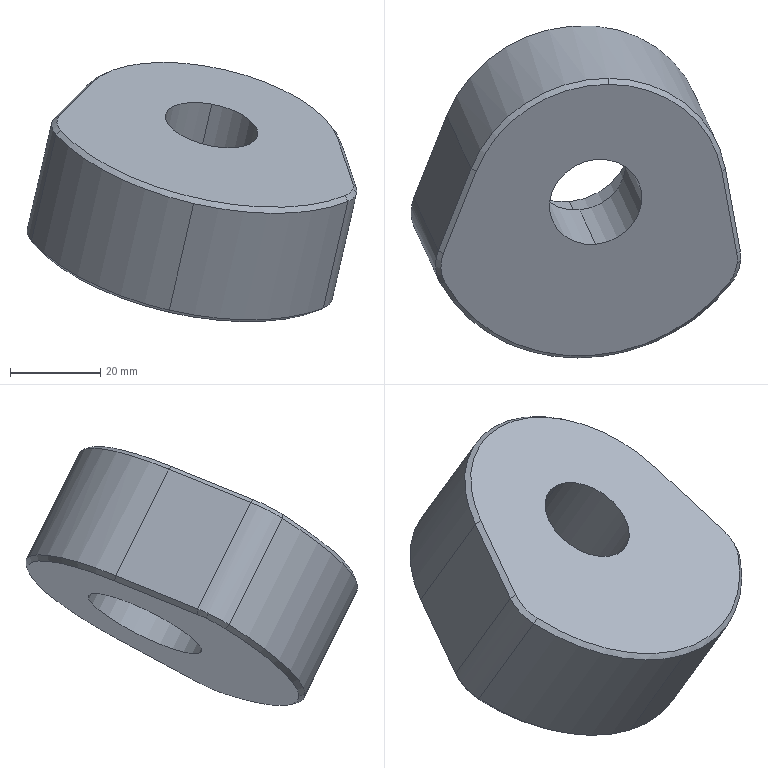Part | SolidWorks | features BaseBody 1 | 1 solid | 31 faces | box 73.281 x 73.868 x 57.617 mm | volume 92633 mm3 | cone 12 | cylinder 10 | plane 9 | commonest cylinder face diameters 20 x3 21 x2 28 x2 78 x2 60 x1
STEP:
#1=CARTESIAN_POINT('',(1948.358,-216.88,907.858));
#2=VERTEX_POINT('',#1);
#3=CARTESIAN_POINT('',(1948.358,-191.807,920.322));
#4=VERTEX_POINT('',#3);
#5=CARTESIAN_POINT('',(1948.358,-204.343,914.09));
#6=DIRECTION('',(-0.2015,0.436,-0.8771));
#7=DIRECTION('',(0.,0.8955,0.4451));
#8=AXIS2_PLACEMENT_3D('',#5,#6,#7);
#9=CIRCLE('',#8,14.);
#10=EDGE_CURVE('',#2,#4,#9,.T.);
#11=ORIENTED_EDGE('',*,*,#10,.T.);
#12=CARTESIAN_POINT('',(1950.674,-196.819,930.404));
#13=VERTEX_POINT('',#12);
#14=CARTESIAN_POINT('',(1946.141,-187.008,910.67));
#15=DIRECTION('',(0.2015,-0.436,0.8771));
#16=VECTOR('',#15,1000.);
#17=LINE('',#14,#16);
#18=EDGE_CURVE('',#4,#13,#17,.T.);
#19=ORIENTED_EDGE('',*,*,#18,.T.);
#20=CARTESIAN_POINT('',(1950.674,-221.892,917.94));
#21=VERTEX_POINT('',#20);
#22=CARTESIAN_POINT('',(1950.674,-209.355,924.172));
#23=DIRECTION('',(-0.2015,0.436,-0.8771));
#24=DIRECTION('',(0.9795,0.08968,-0.1804));
#25=AXIS2_PLACEMENT_3D('',#22,#23,#24);
#26=CIRCLE('',#25,14.);
#27=EDGE_CURVE('',#21,#13,#26,.T.);
#28=ORIENTED_EDGE('',*,*,#27,.F.);
#29=CARTESIAN_POINT('',(1946.141,-212.081,898.206));
#30=DIRECTION('',(0.2015,-0.436,0.8771));
#31=VECTOR('',#30,1000.);
#32=LINE('',#29,#31);
#33=EDGE_CURVE('',#2,#21,#32,.T.);
#34=ORIENTED_EDGE('',*,*,#33,.F.);
#35=EDGE_LOOP('',(#11,#19,#28,#34));
#36=FACE_OUTER_BOUND('',#35,.T.);
#37=CARTESIAN_POINT('',(1946.141,-199.545,904.438));
#38=DIRECTION('',(0.2015,-0.436,0.8771));
#39=DIRECTION('',(0.,-0.8955,-0.4451));
#40=AXIS2_PLACEMENT_3D('',#37,#38,#39);
#41=CYLINDRICAL_SURFACE('',#40,14.);
#42=ADVANCED_FACE('',(#36),#41,.F.);
#43=CARTESIAN_POINT('',(1954.201,-207.585,944.2));
#44=VERTEX_POINT('',#43);
#45=CARTESIAN_POINT('',(1954.201,-226.39,934.852));
#46=VERTEX_POINT('',#45);
#47=CARTESIAN_POINT('',(1954.201,-216.988,939.526));
#48=DIRECTION('',(0.2015,-0.436,0.8771));
#49=DIRECTION('',(0.,-0.8955,-0.4451));
#50=AXIS2_PLACEMENT_3D('',#47,#48,#49);
#51=CIRCLE('',#50,10.5);
#52=EDGE_CURVE('',#44,#46,#51,.T.);
#53=ORIENTED_EDGE('',*,*,#52,.T.);
#54=CARTESIAN_POINT('',(1950.674,-218.758,919.498));
#55=VERTEX_POINT('',#54);
#56=CARTESIAN_POINT('',(1955.207,-228.568,939.233));
#57=DIRECTION('',(-0.2015,0.436,-0.8771));
#58=VECTOR('',#57,1000.);
#59=LINE('',#56,#58);
#60=EDGE_CURVE('',#46,#55,#59,.T.);
#61=ORIENTED_EDGE('',*,*,#60,.T.);
#62=CARTESIAN_POINT('',(1950.674,-199.953,928.846));
#63=VERTEX_POINT('',#62);
#64=CARTESIAN_POINT('',(1950.674,-209.355,924.172));
#65=DIRECTION('',(0.2015,-0.436,0.8771));
#66=DIRECTION('',(0.,0.8955,0.4451));
#67=AXIS2_PLACEMENT_3D('',#64,#65,#66);
#68=CIRCLE('',#67,10.5);
#69=EDGE_CURVE('',#63,#55,#68,.T.);
#70=ORIENTED_EDGE('',*,*,#69,.F.);
#71=CARTESIAN_POINT('',(1955.207,-209.763,948.581));
#72=DIRECTION('',(-0.2015,0.436,-0.8771));
#73=VECTOR('',#72,1000.);
#74=LINE('',#71,#73);
#75=EDGE_CURVE('',#44,#63,#74,.T.);
#76=ORIENTED_EDGE('',*,*,#75,.F.);
#77=EDGE_LOOP('',(#53,#61,#70,#76));
#78=FACE_OUTER_BOUND('',#77,.T.);
#79=CARTESIAN_POINT('',(1955.207,-219.166,943.907));
#80=DIRECTION('',(-0.2015,0.436,-0.8771));
#81=DIRECTION('',(0.,0.8955,0.4451));
#82=AXIS2_PLACEMENT_3D('',#79,#80,#81);
#83=CYLINDRICAL_SURFACE('',#82,10.5);
#84=ADVANCED_FACE('',(#78),#83,.F.);
#85=CARTESIAN_POINT('',(1944.753,-239.877,898.394));
#86=VERTEX_POINT('',#85);
#87=CARTESIAN_POINT('',(1914.132,-223.064,913.786));
#88=VERTEX_POINT('',#87);
#89=CARTESIAN_POINT('',(1948.56,-204.779,914.967));
#90=DIRECTION('',(-0.2015,0.436,-0.8771));
#91=DIRECTION('',(-0.09761,-0.8999,-0.425));
#92=AXIS2_PLACEMENT_3D('',#89,#90,#91);
#93=CIRCLE('',#92,39.);
#94=EDGE_CURVE('',#86,#88,#93,.T.);
#95=ORIENTED_EDGE('',*,*,#94,.F.);
#96=CARTESIAN_POINT('',(1950.193,-251.649,922.076));
#97=VERTEX_POINT('',#96);
#98=CARTESIAN_POINT('',(1944.644,-239.641,897.921));
#99=DIRECTION('',(0.2015,-0.436,0.8771));
#100=VECTOR('',#99,1000.);
#101=LINE('',#98,#100);
#102=EDGE_CURVE('',#86,#97,#101,.T.);
#103=ORIENTED_EDGE('',*,*,#102,.T.);
#104=CARTESIAN_POINT('',(1919.572,-234.836,937.467));
#105=VERTEX_POINT('',#104);
#106=CARTESIAN_POINT('',(1953.999,-216.552,938.649));
#107=DIRECTION('',(0.2015,-0.436,0.8771));
#108=DIRECTION('',(0.09761,0.8999,0.425));
#109=AXIS2_PLACEMENT_3D('',#106,#107,#108);
#110=CIRCLE('',#109,39.);
#111=EDGE_CURVE('',#105,#97,#110,.T.);
#112=ORIENTED_EDGE('',*,*,#111,.F.);
#113=CARTESIAN_POINT('',(1914.023,-222.829,913.312));
#114=DIRECTION('',(-0.2015,0.436,-0.8771));
#115=VECTOR('',#114,1000.);
#116=LINE('',#113,#115);
#117=EDGE_CURVE('',#105,#88,#116,.T.);
#118=ORIENTED_EDGE('',*,*,#117,.T.);
#119=EDGE_LOOP('',(#95,#103,#112,#118));
#120=FACE_OUTER_BOUND('',#119,.T.);
#121=CARTESIAN_POINT('',(1948.451,-204.544,914.494));
#122=DIRECTION('',(0.2015,-0.436,0.8771));
#123=DIRECTION('',(-0.09761,-0.8999,-0.425));
#124=AXIS2_PLACEMENT_3D('',#121,#122,#123);
#125=CYLINDRICAL_SURFACE('',#124,39.);
#126=ADVANCED_FACE('',(#120),#125,.T.);
#127=CARTESIAN_POINT('',(1986.396,-230.148,924.449));
#128=VERTEX_POINT('',#127);
#129=CARTESIAN_POINT('',(1986.317,-227.819,925.625));
#130=VERTEX_POINT('',#129);
#131=CARTESIAN_POINT('',(1976.65,-230.148,926.687));
#132=DIRECTION('',(0.2015,-0.436,0.8771));
#133=DIRECTION('',(0.9746,0.,-0.2239));
#134=AXIS2_PLACEMENT_3D('',#131,#132,#133);
#135=CIRCLE('',#134,10.);
#136=EDGE_CURVE('',#128,#130,#135,.T.);
#137=ORIENTED_EDGE('',*,*,#136,.F.);
#138=CARTESIAN_POINT('',(1980.957,-218.375,900.766));
#139=VERTEX_POINT('',#138);
#140=CARTESIAN_POINT('',(1986.505,-230.384,924.922));
#141=DIRECTION('',(-0.2015,0.436,-0.8771));
#142=VECTOR('',#141,1000.);
#143=LINE('',#140,#142);
#144=EDGE_CURVE('',#128,#139,#143,.T.);
#145=ORIENTED_EDGE('',*,*,#144,.T.);
#146=CARTESIAN_POINT('',(1980.877,-216.046,901.943));
#147=VERTEX_POINT('',#146);
#148=CARTESIAN_POINT('',(1971.21,-218.375,903.005));
#149=DIRECTION('',(-0.2015,0.436,-0.8771));
#150=DIRECTION('',(-0.9746,0.,0.2239));
#151=AXIS2_PLACEMENT_3D('',#148,#149,#150);
#152=CIRCLE('',#151,10.);
#153=EDGE_CURVE('',#147,#139,#152,.T.);
#154=ORIENTED_EDGE('',*,*,#153,.F.);
#155=CARTESIAN_POINT('',(1980.768,-215.811,901.469));
#156=DIRECTION('',(-0.2015,0.436,-0.8771));
#157=VECTOR('',#156,1000.);
#158=LINE('',#155,#157);
#159=EDGE_CURVE('',#130,#147,#158,.T.);
#160=ORIENTED_EDGE('',*,*,#159,.F.);
#161=EDGE_LOOP('',(#137,#145,#154,#160));
#162=FACE_OUTER_BOUND('',#161,.T.);
#163=CARTESIAN_POINT('',(1976.759,-230.384,927.161));
#164=DIRECTION('',(-0.2015,0.436,-0.8771));
#165=DIRECTION('',(0.9746,0.,-0.2239));
#166=AXIS2_PLACEMENT_3D('',#163,#164,#165);
#167=CYLINDRICAL_SURFACE('',#166,10.);
#168=ADVANCED_FACE('',(#162),#167,.T.);
#169=CARTESIAN_POINT('',(1957.032,-190.89,951.85));
#170=VERTEX_POINT('',#169);
#171=CARTESIAN_POINT('',(1927.633,-210.233,948.986));
#172=VERTEX_POINT('',#171);
#173=CARTESIAN_POINT('',(1954.201,-216.988,939.526));
#174=DIRECTION('',(0.2015,-0.436,0.8771));
#175=DIRECTION('',(0.9667,0.2329,-0.1063));
#176=AXIS2_PLACEMENT_3D('',#173,#174,#175);
#177=CIRCLE('',#176,29.);
#178=EDGE_CURVE('',#170,#172,#177,.T.);
#179=ORIENTED_EDGE('',*,*,#178,.F.);
#180=CARTESIAN_POINT('',(1956.928,-189.554,951.397));
#181=VERTEX_POINT('',#180);
#182=CARTESIAN_POINT('',(1957.04,-191.003,951.888));
#183=DIRECTION('',(-0.07344,0.9447,-0.3197));
#184=VECTOR('',#183,1000.);
#185=LINE('',#182,#184);
#186=EDGE_CURVE('',#170,#181,#185,.T.);
#187=ORIENTED_EDGE('',*,*,#186,.T.);
#188=CARTESIAN_POINT('',(1926.515,-209.564,948.436));
#189=VERTEX_POINT('',#188);
#190=CARTESIAN_POINT('',(1953.999,-216.552,938.649));
#191=DIRECTION('',(0.2015,-0.436,0.8771));
#192=DIRECTION('',(0.09761,0.8999,0.425));
#193=AXIS2_PLACEMENT_3D('',#190,#191,#192);
#194=CIRCLE('',#193,30.);
#195=EDGE_CURVE('',#181,#189,#194,.T.);
#196=ORIENTED_EDGE('',*,*,#195,.T.);
#197=CARTESIAN_POINT('',(1927.633,-210.233,948.986));
#198=DIRECTION('',(-0.7903,0.473,-0.3895));
#199=VECTOR('',#198,1000.);
#200=LINE('',#197,#199);
#201=EDGE_CURVE('',#172,#189,#200,.T.);
#202=ORIENTED_EDGE('',*,*,#201,.F.);
#203=EDGE_LOOP('',(#179,#187,#196,#202));
#204=FACE_OUTER_BOUND('',#203,.T.);
#205=CARTESIAN_POINT('',(1954.218,-217.025,939.6));
#206=DIRECTION('',(-0.2015,0.436,-0.8771));
#207=DIRECTION('',(0.09761,0.8999,0.425));
#208=AXIS2_PLACEMENT_3D('',#205,#206,#207);
#209=CONICAL_SURFACE('',#208,28.915,0.7854);
#210=ADVANCED_FACE('',(#204),#209,.T.);
#211=CARTESIAN_POINT('',(1985.624,-230.584,925.549));
#212=VERTEX_POINT('',#211);
#213=CARTESIAN_POINT('',(1985.552,-228.488,926.608));
#214=VERTEX_POINT('',#213);
#215=CARTESIAN_POINT('',(1976.852,-230.584,927.564));
#216=DIRECTION('',(0.2015,-0.436,0.8771));
#217=DIRECTION('',(0.9746,0.,-0.2239));
#218=AXIS2_PLACEMENT_3D('',#215,#216,#217);
#219=CIRCLE('',#218,9.);
#220=EDGE_CURVE('',#212,#214,#219,.T.);
#221=ORIENTED_EDGE('',*,*,#220,.F.);
#222=CARTESIAN_POINT('',(1985.558,-230.621,925.643));
#223=DIRECTION('',(0.5467,0.3083,-0.7785));
#224=VECTOR('',#223,1000.);
#225=LINE('',#222,#224);
#226=EDGE_CURVE('',#212,#128,#225,.T.);
#227=ORIENTED_EDGE('',*,*,#226,.T.);
#228=ORIENTED_EDGE('',*,*,#136,.T.);
#229=CARTESIAN_POINT('',(1985.552,-228.488,926.608));
#230=CARTESIAN_POINT('',(1985.807,-228.265,926.28));
#231=CARTESIAN_POINT('',(1986.062,-228.042,925.952));
#232=CARTESIAN_POINT('',(1986.317,-227.819,925.625));
#233=B_SPLINE_CURVE_WITH_KNOTS('',3,(#229,#230,#231,#232),.UNSPECIFIED.,.F.,.F.,(4,4),(0.,1.),.UNSPECIFIED.);
#234=EDGE_CURVE('',#214,#130,#233,.T.);
#235=ORIENTED_EDGE('',*,*,#234,.F.);
#236=EDGE_LOOP('',(#221,#227,#228,#235));
#237=FACE_OUTER_BOUND('',#236,.T.);
#238=CARTESIAN_POINT('',(1976.869,-230.621,927.639));
#239=DIRECTION('',(-0.2015,0.436,-0.8771));
#240=DIRECTION('',(0.9746,0.,-0.2239));
#241=AXIS2_PLACEMENT_3D('',#238,#239,#240);
#242=CONICAL_SURFACE('',#241,8.915,0.7854);
#243=ADVANCED_FACE('',(#237),#242,.T.);
#244=CARTESIAN_POINT('',(1913.986,-217.94,915.226));
#245=VERTEX_POINT('',#244);
#246=CARTESIAN_POINT('',(1914.513,-215.843,916.148));
#247=VERTEX_POINT('',#246);
#248=CARTESIAN_POINT('',(1922.758,-217.94,913.212));
#249=DIRECTION('',(-0.2015,0.436,-0.8771));
#250=DIRECTION('',(-0.9746,0.,0.2239));
#251=AXIS2_PLACEMENT_3D('',#248,#249,#250);
#252=CIRCLE('',#251,9.);
#253=EDGE_CURVE('',#245,#247,#252,.T.);
#254=ORIENTED_EDGE('',*,*,#253,.F.);
#255=CARTESIAN_POINT('',(1913.213,-218.375,916.327));
#256=VERTEX_POINT('',#255);
#257=CARTESIAN_POINT('',(1914.052,-217.903,915.133));
#258=DIRECTION('',(-0.5467,-0.3083,0.7785));
#259=VECTOR('',#258,1000.);
#260=LINE('',#257,#259);
#261=EDGE_CURVE('',#245,#256,#260,.T.);
#262=ORIENTED_EDGE('',*,*,#261,.T.);
#263=CARTESIAN_POINT('',(1913.798,-216.046,917.351));
#264=VERTEX_POINT('',#263);
#265=CARTESIAN_POINT('',(1922.96,-218.375,914.088));
#266=DIRECTION('',(-0.2015,0.436,-0.8771));
#267=DIRECTION('',(-0.9746,0.,0.2239));
#268=AXIS2_PLACEMENT_3D('',#265,#266,#267);
#269=CIRCLE('',#268,10.);
#270=EDGE_CURVE('',#256,#264,#269,.T.);
#271=ORIENTED_EDGE('',*,*,#270,.T.);
#272=CARTESIAN_POINT('',(1914.513,-215.843,916.148));
#273=CARTESIAN_POINT('',(1914.275,-215.911,916.549));
#274=CARTESIAN_POINT('',(1914.036,-215.979,916.95));
#275=CARTESIAN_POINT('',(1913.798,-216.046,917.351));
#276=B_SPLINE_CURVE_WITH_KNOTS('',3,(#272,#273,#274,#275),.UNSPECIFIED.,.F.,.F.,(4,4),(0.,1.),.UNSPECIFIED.);
#277=EDGE_CURVE('',#247,#264,#276,.T.);
#278=ORIENTED_EDGE('',*,*,#277,.F.);
#279=EDGE_LOOP('',(#254,#262,#271,#278));
#280=FACE_OUTER_BOUND('',#279,.T.);
#281=CARTESIAN_POINT('',(1922.741,-217.903,913.137));
#282=DIRECTION('',(0.2015,-0.436,0.8771));
#283=DIRECTION('',(-0.9746,0.,0.2239));
#284=AXIS2_PLACEMENT_3D('',#281,#282,#283);
#285=CONICAL_SURFACE('',#284,8.915,0.7854);
#286=ADVANCED_FACE('',(#280),#285,.T.);
#287=CARTESIAN_POINT('',(1944.649,-238.541,897.942));
#288=VERTEX_POINT('',#287);
#289=CARTESIAN_POINT('',(1914.813,-222.159,912.939));
#290=VERTEX_POINT('',#289);
#291=CARTESIAN_POINT('',(1948.358,-204.343,914.09));
#292=DIRECTION('',(-0.2015,0.436,-0.8771));
#293=DIRECTION('',(-0.09761,-0.8999,-0.425));
#294=AXIS2_PLACEMENT_3D('',#291,#292,#293);
#295=CIRCLE('',#294,38.);
#296=EDGE_CURVE('',#288,#290,#295,.T.);
#297=ORIENTED_EDGE('',*,*,#296,.F.);
#298=CARTESIAN_POINT('',(1944.64,-238.428,897.904));
#299=DIRECTION('',(0.07344,-0.9447,0.3197));
#300=VECTOR('',#299,1000.);
#301=LINE('',#298,#300);
#302=EDGE_CURVE('',#288,#86,#301,.T.);
#303=ORIENTED_EDGE('',*,*,#302,.T.);
#304=ORIENTED_EDGE('',*,*,#94,.T.);
#305=CARTESIAN_POINT('',(1914.813,-222.159,912.939));
#306=CARTESIAN_POINT('',(1914.586,-222.461,913.221));
#307=CARTESIAN_POINT('',(1914.359,-222.762,913.503));
#308=CARTESIAN_POINT('',(1914.132,-223.064,913.786));
#309=B_SPLINE_CURVE_WITH_KNOTS('',3,(#305,#306,#307,#308),.UNSPECIFIED.,.F.,.F.,(4,4),(0.,1.),.UNSPECIFIED.);
#310=EDGE_CURVE('',#290,#88,#309,.T.);
#311=ORIENTED_EDGE('',*,*,#310,.F.);
#312=EDGE_LOOP('',(#297,#303,#304,#311));
#313=FACE_OUTER_BOUND('',#312,.T.);
#314=CARTESIAN_POINT('',(1948.341,-204.306,914.016));
#315=DIRECTION('',(0.2015,-0.436,0.8771));
#316=DIRECTION('',(-0.09761,-0.8999,-0.425));
#317=AXIS2_PLACEMENT_3D('',#314,#315,#316);
#318=CONICAL_SURFACE('',#317,37.915,0.7854);
#319=ADVANCED_FACE('',(#313),#318,.T.);
#320=CARTESIAN_POINT('',(1921.79,-197.589,923.551));
#321=VERTEX_POINT('',#320);
#322=CARTESIAN_POINT('',(1976.392,-197.589,911.009));
#323=VERTEX_POINT('',#322);
#324=CARTESIAN_POINT('',(1948.358,-204.343,914.09));
#325=DIRECTION('',(-0.2015,0.436,-0.8771));
#326=DIRECTION('',(-0.9161,0.2329,0.3262));
#327=AXIS2_PLACEMENT_3D('',#324,#325,#326);
#328=CIRCLE('',#327,29.);
#329=EDGE_CURVE('',#321,#323,#328,.T.);
#330=ORIENTED_EDGE('',*,*,#329,.T.);
#331=CARTESIAN_POINT('',(1979.709,-215.843,901.172));
#332=VERTEX_POINT('',#331);
#333=CARTESIAN_POINT('',(1976.392,-197.589,911.009));
#334=DIRECTION('',(0.158,-0.8693,-0.4684));
#335=VECTOR('',#334,1000.);
#336=LINE('',#333,#335);
#337=EDGE_CURVE('',#323,#332,#336,.T.);
#338=ORIENTED_EDGE('',*,*,#337,.T.);
#339=CARTESIAN_POINT('',(1978.039,-222.159,898.416));
#340=VERTEX_POINT('',#339);
#341=CARTESIAN_POINT('',(1971.009,-217.94,902.128));
#342=DIRECTION('',(-0.2015,0.436,-0.8771));
#343=DIRECTION('',(-0.9746,0.,0.2239));
#344=AXIS2_PLACEMENT_3D('',#341,#342,#343);
#345=CIRCLE('',#344,9.);
#346=EDGE_CURVE('',#332,#340,#345,.T.);
#347=ORIENTED_EDGE('',*,*,#346,.T.);
#348=CARTESIAN_POINT('',(1948.358,-204.343,914.09));
#349=DIRECTION('',(-0.2015,0.436,-0.8771));
#350=DIRECTION('',(-0.09761,-0.8999,-0.425));
#351=AXIS2_PLACEMENT_3D('',#348,#349,#350);
#352=CIRCLE('',#351,38.);
#353=EDGE_CURVE('',#340,#288,#352,.T.);
#354=ORIENTED_EDGE('',*,*,#353,.T.);
#355=ORIENTED_EDGE('',*,*,#296,.T.);
#356=CARTESIAN_POINT('',(1922.758,-217.94,913.212));
#357=DIRECTION('',(-0.2015,0.436,-0.8771));
#358=DIRECTION('',(-0.9746,0.,0.2239));
#359=AXIS2_PLACEMENT_3D('',#356,#357,#358);
#360=CIRCLE('',#359,9.);
#361=EDGE_CURVE('',#290,#245,#360,.T.);
#362=ORIENTED_EDGE('',*,*,#361,.T.);
#363=ORIENTED_EDGE('',*,*,#253,.T.);
#364=CARTESIAN_POINT('',(1914.513,-215.843,916.148));
#365=DIRECTION('',(0.3465,0.8693,0.3525));
#366=VECTOR('',#365,1000.);
#367=LINE('',#364,#366);
#368=EDGE_CURVE('',#247,#321,#367,.T.);
#369=ORIENTED_EDGE('',*,*,#368,.T.);
#370=EDGE_LOOP('',(#330,#338,#347,#354,#355,#362,#363,#369));
#371=FACE_OUTER_BOUND('',#370,.T.);
#372=ORIENTED_EDGE('',*,*,#10,.F.);
#373=CARTESIAN_POINT('',(1948.358,-204.343,914.09));
#374=DIRECTION('',(-0.2015,0.436,-0.8771));
#375=DIRECTION('',(0.,0.8955,0.4451));
#376=AXIS2_PLACEMENT_3D('',#373,#374,#375);
#377=CIRCLE('',#376,14.);
#378=EDGE_CURVE('',#4,#2,#377,.T.);
#379=ORIENTED_EDGE('',*,*,#378,.F.);
#380=EDGE_LOOP('',(#372,#379));
#381=FACE_BOUND('',#380,.T.);
#382=CARTESIAN_POINT('',(1910.301,-239.747,905.232));
#383=DIRECTION('',(-0.2015,0.436,-0.8771));
#384=DIRECTION('',(0.09761,0.8999,0.425));
#385=AXIS2_PLACEMENT_3D('',#382,#383,#384);
#386=PLANE('',#385);
#387=ADVANCED_FACE('',(#371,#381),#386,.T.);
#388=ORIENTED_EDGE('',*,*,#277,.T.);
#389=CARTESIAN_POINT('',(1921.075,-197.792,924.754));
#390=VERTEX_POINT('',#389);
#391=CARTESIAN_POINT('',(1913.798,-216.046,917.351));
#392=DIRECTION('',(0.3465,0.8693,0.3525));
#393=VECTOR('',#392,1000.);
#394=LINE('',#391,#393);
#395=EDGE_CURVE('',#264,#390,#394,.T.);
#396=ORIENTED_EDGE('',*,*,#395,.T.);
#397=CARTESIAN_POINT('',(1921.79,-197.589,923.551));
#398=DIRECTION('',(-0.5054,-0.1436,0.8509));
#399=VECTOR('',#398,1000.);
#400=LINE('',#397,#399);
#401=EDGE_CURVE('',#321,#390,#400,.T.);
#402=ORIENTED_EDGE('',*,*,#401,.F.);
#403=ORIENTED_EDGE('',*,*,#368,.F.);
#404=EDGE_LOOP('',(#388,#396,#402,#403));
#405=FACE_OUTER_BOUND('',#404,.T.);
#406=CARTESIAN_POINT('',(1913.563,-216.646,917.099));
#407=DIRECTION('',(-0.7903,0.473,-0.3895));
#408=DIRECTION('',(0.2464,0.8273,0.5048));
#409=AXIS2_PLACEMENT_3D('',#406,#407,#408);
#410=PLANE('',#409);
#411=ADVANCED_FACE('',(#405),#410,.T.);
#412=ORIENTED_EDGE('',*,*,#401,.T.);
#413=CARTESIAN_POINT('',(1977.56,-197.792,911.78));
#414=VERTEX_POINT('',#413);
#415=CARTESIAN_POINT('',(1948.56,-204.779,914.967));
#416=DIRECTION('',(-0.2015,0.436,-0.8771));
#417=DIRECTION('',(-0.09761,-0.8999,-0.425));
#418=AXIS2_PLACEMENT_3D('',#415,#416,#417);
#419=CIRCLE('',#418,30.);
#420=EDGE_CURVE('',#390,#414,#419,.T.);
#421=ORIENTED_EDGE('',*,*,#420,.T.);
#422=CARTESIAN_POINT('',(1976.392,-197.589,911.009));
#423=DIRECTION('',(0.826,-0.1436,0.5451));
#424=VECTOR('',#423,1000.);
#425=LINE('',#422,#424);
#426=EDGE_CURVE('',#323,#414,#425,.T.);
#427=ORIENTED_EDGE('',*,*,#426,.F.);
#428=ORIENTED_EDGE('',*,*,#329,.F.);
#429=EDGE_LOOP('',(#412,#421,#427,#428));
#430=FACE_OUTER_BOUND('',#429,.T.);
#431=CARTESIAN_POINT('',(1948.341,-204.306,914.016));
#432=DIRECTION('',(0.2015,-0.436,0.8771));
#433=DIRECTION('',(-0.09761,-0.8999,-0.425));
#434=AXIS2_PLACEMENT_3D('',#431,#432,#433);
#435=CONICAL_SURFACE('',#434,28.915,0.7854);
#436=ADVANCED_FACE('',(#430),#435,.T.);
#437=ORIENTED_EDGE('',*,*,#426,.T.);
#438=CARTESIAN_POINT('',(1977.56,-197.792,911.78));
#439=DIRECTION('',(0.158,-0.8693,-0.4684));
#440=VECTOR('',#439,1000.);
#441=LINE('',#438,#440);
#442=EDGE_CURVE('',#414,#147,#441,.T.);
#443=ORIENTED_EDGE('',*,*,#442,.T.);
#444=CARTESIAN_POINT('',(1979.709,-215.843,901.172));
#445=CARTESIAN_POINT('',(1980.099,-215.911,901.429));
#446=CARTESIAN_POINT('',(1980.488,-215.979,901.686));
#447=CARTESIAN_POINT('',(1980.877,-216.046,901.943));
#448=B_SPLINE_CURVE_WITH_KNOTS('',3,(#444,#445,#446,#447),.UNSPECIFIED.,.F.,.F.,(4,4),(0.,1.),.UNSPECIFIED.);
#449=EDGE_CURVE('',#332,#147,#448,.T.);
#450=ORIENTED_EDGE('',*,*,#449,.F.);
#451=ORIENTED_EDGE('',*,*,#337,.F.);
#452=EDGE_LOOP('',(#437,#443,#450,#451));
#453=FACE_OUTER_BOUND('',#452,.T.);
#454=CARTESIAN_POINT('',(1976.321,-214.969,899.131));
#455=DIRECTION('',(0.5411,0.473,-0.6953));
#456=DIRECTION('',(-0.001439,0.8273,0.5617));
#457=AXIS2_PLACEMENT_3D('',#454,#455,#456);
#458=PLANE('',#457);
#459=ADVANCED_FACE('',(#453),#458,.T.);
#460=ORIENTED_EDGE('',*,*,#449,.T.);
#461=ORIENTED_EDGE('',*,*,#153,.T.);
#462=CARTESIAN_POINT('',(1979.021,-223.064,898.881));
#463=VERTEX_POINT('',#462);
#464=CARTESIAN_POINT('',(1971.21,-218.375,903.005));
#465=DIRECTION('',(-0.2015,0.436,-0.8771));
#466=DIRECTION('',(-0.9746,0.,0.2239));
#467=AXIS2_PLACEMENT_3D('',#464,#465,#466);
#468=CIRCLE('',#467,10.);
#469=EDGE_CURVE('',#139,#463,#468,.T.);
#470=ORIENTED_EDGE('',*,*,#469,.T.);
#471=CARTESIAN_POINT('',(1978.039,-222.159,898.416));
#472=CARTESIAN_POINT('',(1978.366,-222.461,898.571));
#473=CARTESIAN_POINT('',(1978.694,-222.762,898.726));
#474=CARTESIAN_POINT('',(1979.021,-223.064,898.881));
#475=B_SPLINE_CURVE_WITH_KNOTS('',3,(#471,#472,#473,#474),.UNSPECIFIED.,.F.,.F.,(4,4),(0.,1.),.UNSPECIFIED.);
#476=EDGE_CURVE('',#340,#463,#475,.T.);
#477=ORIENTED_EDGE('',*,*,#476,.F.);
#478=ORIENTED_EDGE('',*,*,#346,.F.);
#479=EDGE_LOOP('',(#460,#461,#470,#477,#478));
#480=FACE_OUTER_BOUND('',#479,.T.);
#481=CARTESIAN_POINT('',(1970.992,-217.903,902.054));
#482=DIRECTION('',(0.2015,-0.436,0.8771));
#483=DIRECTION('',(-0.9746,0.,0.2239));
#484=AXIS2_PLACEMENT_3D('',#481,#482,#483);
#485=CONICAL_SURFACE('',#484,8.915,0.7854);
#486=ADVANCED_FACE('',(#480),#485,.T.);
#487=ORIENTED_EDGE('',*,*,#302,.F.);
#488=ORIENTED_EDGE('',*,*,#353,.F.);
#489=ORIENTED_EDGE('',*,*,#476,.T.);
#490=CARTESIAN_POINT('',(1948.56,-204.779,914.967));
#491=DIRECTION('',(-0.2015,0.436,-0.8771));
#492=DIRECTION('',(-0.09761,-0.8999,-0.425));
#493=AXIS2_PLACEMENT_3D('',#490,#491,#492);
#494=CIRCLE('',#493,39.);
#495=EDGE_CURVE('',#463,#86,#494,.T.);
#496=ORIENTED_EDGE('',*,*,#495,.T.);
#497=EDGE_LOOP('',(#487,#488,#489,#496));
#498=FACE_OUTER_BOUND('',#497,.T.);
#499=CARTESIAN_POINT('',(1948.341,-204.306,914.016));
#500=DIRECTION('',(0.2015,-0.436,0.8771));
#501=DIRECTION('',(-0.09761,-0.8999,-0.425));
#502=AXIS2_PLACEMENT_3D('',#499,#500,#501);
#503=CONICAL_SURFACE('',#502,37.915,0.7854);
#504=ADVANCED_FACE('',(#498),#503,.T.);
#505=ORIENTED_EDGE('',*,*,#261,.F.);
#506=ORIENTED_EDGE('',*,*,#361,.F.);
#507=ORIENTED_EDGE('',*,*,#310,.T.);
#508=CARTESIAN_POINT('',(1922.96,-218.375,914.088));
#509=DIRECTION('',(-0.2015,0.436,-0.8771));
#510=DIRECTION('',(-0.9746,0.,0.2239));
#511=AXIS2_PLACEMENT_3D('',#508,#509,#510);
#512=CIRCLE('',#511,10.);
#513=EDGE_CURVE('',#88,#256,#512,.T.);
#514=ORIENTED_EDGE('',*,*,#513,.T.);
#515=EDGE_LOOP('',(#505,#506,#507,#514));
#516=FACE_OUTER_BOUND('',#515,.T.);
#517=CARTESIAN_POINT('',(1922.741,-217.903,913.137));
#518=DIRECTION('',(0.2015,-0.436,0.8771));
#519=DIRECTION('',(-0.9746,0.,0.2239));
#520=AXIS2_PLACEMENT_3D('',#517,#518,#519);
#521=CONICAL_SURFACE('',#520,8.915,0.7854);
#522=ADVANCED_FACE('',(#516),#521,.T.);
#523=CARTESIAN_POINT('',(1919.238,-227.819,941.033));
#524=VERTEX_POINT('',#523);
#525=CARTESIAN_POINT('',(1919.347,-228.054,941.506));
#526=DIRECTION('',(-0.2015,0.436,-0.8771));
#527=VECTOR('',#526,1000.);
#528=LINE('',#525,#527);
#529=EDGE_CURVE('',#524,#264,#528,.T.);
#530=ORIENTED_EDGE('',*,*,#529,.T.);
#531=ORIENTED_EDGE('',*,*,#270,.F.);
#532=ORIENTED_EDGE('',*,*,#513,.F.);
#533=ORIENTED_EDGE('',*,*,#117,.F.);
#534=CARTESIAN_POINT('',(1928.399,-230.148,937.771));
#535=DIRECTION('',(0.2015,-0.436,0.8771));
#536=DIRECTION('',(0.9746,0.,-0.2239));
#537=AXIS2_PLACEMENT_3D('',#534,#535,#536);
#538=CIRCLE('',#537,10.);
#539=EDGE_CURVE('',#524,#105,#538,.T.);
#540=ORIENTED_EDGE('',*,*,#539,.F.);
#541=EDGE_LOOP('',(#530,#531,#532,#533,#540));
#542=FACE_OUTER_BOUND('',#541,.T.);
#543=CARTESIAN_POINT('',(1928.508,-230.384,938.244));
#544=DIRECTION('',(-0.2015,0.436,-0.8771));
#545=DIRECTION('',(0.9746,0.,-0.2239));
#546=AXIS2_PLACEMENT_3D('',#543,#544,#545);
#547=CYLINDRICAL_SURFACE('',#546,10.);
#548=ADVANCED_FACE('',(#542),#547,.T.);
#549=CARTESIAN_POINT('',(1920.355,-228.488,941.583));
#550=VERTEX_POINT('',#549);
#551=CARTESIAN_POINT('',(1920.355,-228.488,941.583));
#552=CARTESIAN_POINT('',(1919.983,-228.265,941.4));
#553=CARTESIAN_POINT('',(1919.61,-228.042,941.216));
#554=CARTESIAN_POINT('',(1919.238,-227.819,941.033));
#555=B_SPLINE_CURVE_WITH_KNOTS('',3,(#551,#552,#553,#554),.UNSPECIFIED.,.F.,.F.,(4,4),(0.,1.),.UNSPECIFIED.);
#556=EDGE_CURVE('',#550,#524,#555,.T.);
#557=ORIENTED_EDGE('',*,*,#556,.T.);
#558=ORIENTED_EDGE('',*,*,#539,.T.);
#559=CARTESIAN_POINT('',(1920.656,-234.804,938.375));
#560=VERTEX_POINT('',#559);
#561=CARTESIAN_POINT('',(1920.656,-234.804,938.375));
#562=CARTESIAN_POINT('',(1920.294,-234.814,938.072));
#563=CARTESIAN_POINT('',(1919.933,-234.825,937.77));
#564=CARTESIAN_POINT('',(1919.572,-234.836,937.467));
#565=B_SPLINE_CURVE_WITH_KNOTS('',3,(#561,#562,#563,#564),.UNSPECIFIED.,.F.,.F.,(4,4),(0.,1.),.UNSPECIFIED.);
#566=EDGE_CURVE('',#560,#105,#565,.T.);
#567=ORIENTED_EDGE('',*,*,#566,.F.);
#568=CARTESIAN_POINT('',(1928.601,-230.584,938.647));
#569=DIRECTION('',(0.2015,-0.436,0.8771));
#570=DIRECTION('',(0.9746,0.,-0.2239));
#571=AXIS2_PLACEMENT_3D('',#568,#569,#570);
#572=CIRCLE('',#571,9.);
#573=EDGE_CURVE('',#550,#560,#572,.T.);
#574=ORIENTED_EDGE('',*,*,#573,.F.);
#575=EDGE_LOOP('',(#557,#558,#567,#574));
#576=FACE_OUTER_BOUND('',#575,.T.);
#577=CARTESIAN_POINT('',(1928.618,-230.621,938.722));
#578=DIRECTION('',(-0.2015,0.436,-0.8771));
#579=DIRECTION('',(0.9746,0.,-0.2239));
#580=AXIS2_PLACEMENT_3D('',#577,#578,#579);
#581=CONICAL_SURFACE('',#580,8.915,0.7854);
#582=ADVANCED_FACE('',(#576),#581,.T.);
#583=ORIENTED_EDGE('',*,*,#52,.F.);
#584=CARTESIAN_POINT('',(1954.201,-216.988,939.526));
#585=DIRECTION('',(0.2015,-0.436,0.8771));
#586=DIRECTION('',(0.,-0.8955,-0.4451));
#587=AXIS2_PLACEMENT_3D('',#584,#585,#586);
#588=CIRCLE('',#587,10.5);
#589=EDGE_CURVE('',#46,#44,#588,.T.);
#590=ORIENTED_EDGE('',*,*,#589,.F.);
#591=EDGE_LOOP('',(#583,#590));
#592=FACE_BOUND('',#591,.T.);
#593=CARTESIAN_POINT('',(1982.234,-210.233,936.445));
#594=VERTEX_POINT('',#593);
#595=CARTESIAN_POINT('',(1985.552,-228.488,926.608));
#596=DIRECTION('',(-0.158,0.8693,0.4684));
#597=VECTOR('',#596,1000.);
#598=LINE('',#595,#597);
#599=EDGE_CURVE('',#214,#594,#598,.T.);
#600=ORIENTED_EDGE('',*,*,#599,.T.);
#601=CARTESIAN_POINT('',(1954.201,-216.988,939.526));
#602=DIRECTION('',(0.2015,-0.436,0.8771));
#603=DIRECTION('',(0.9667,0.2329,-0.1063));
#604=AXIS2_PLACEMENT_3D('',#601,#602,#603);
#605=CIRCLE('',#604,29.);
#606=EDGE_CURVE('',#594,#170,#605,.T.);
#607=ORIENTED_EDGE('',*,*,#606,.T.);
#608=ORIENTED_EDGE('',*,*,#178,.T.);
#609=CARTESIAN_POINT('',(1927.633,-210.233,948.986));
#610=DIRECTION('',(-0.3465,-0.8693,-0.3525));
#611=VECTOR('',#610,1000.);
#612=LINE('',#609,#611);
#613=EDGE_CURVE('',#172,#550,#612,.T.);
#614=ORIENTED_EDGE('',*,*,#613,.T.);
#615=ORIENTED_EDGE('',*,*,#573,.T.);
#616=CARTESIAN_POINT('',(1983.881,-234.804,923.852));
#617=VERTEX_POINT('',#616);
#618=CARTESIAN_POINT('',(1954.201,-216.988,939.526));
#619=DIRECTION('',(0.2015,-0.436,0.8771));
#620=DIRECTION('',(-0.09761,-0.8999,-0.425));
#621=AXIS2_PLACEMENT_3D('',#618,#619,#620);
#622=CIRCLE('',#621,38.);
#623=EDGE_CURVE('',#560,#617,#622,.T.);
#624=ORIENTED_EDGE('',*,*,#623,.T.);
#625=CARTESIAN_POINT('',(1976.852,-230.584,927.564));
#626=DIRECTION('',(0.2015,-0.436,0.8771));
#627=DIRECTION('',(0.9746,0.,-0.2239));
#628=AXIS2_PLACEMENT_3D('',#625,#626,#627);
#629=CIRCLE('',#628,9.);
#630=EDGE_CURVE('',#617,#212,#629,.T.);
#631=ORIENTED_EDGE('',*,*,#630,.T.);
#632=ORIENTED_EDGE('',*,*,#220,.T.);
#633=EDGE_LOOP('',(#600,#607,#608,#614,#615,#624,#631,#632));
#634=FACE_OUTER_BOUND('',#633,.T.);
#635=CARTESIAN_POINT('',(1916.143,-252.392,930.668));
#636=DIRECTION('',(0.2015,-0.436,0.8771));
#637=DIRECTION('',(0.9746,0.,-0.2239));
#638=AXIS2_PLACEMENT_3D('',#635,#636,#637);
#639=PLANE('',#638);
#640=ADVANCED_FACE('',(#592,#634),#639,.T.);
#641=ORIENTED_EDGE('',*,*,#226,.F.);
#642=ORIENTED_EDGE('',*,*,#630,.F.);
#643=CARTESIAN_POINT('',(1984.461,-234.836,922.562));
#644=VERTEX_POINT('',#643);
#645=CARTESIAN_POINT('',(1983.881,-234.804,923.852));
#646=CARTESIAN_POINT('',(1984.075,-234.815,923.422));
#647=CARTESIAN_POINT('',(1984.268,-234.826,922.992));
#648=CARTESIAN_POINT('',(1984.461,-234.836,922.562));
#649=B_SPLINE_CURVE_WITH_KNOTS('',3,(#645,#646,#647,#648),.UNSPECIFIED.,.F.,.F.,(4,4),(0.,1.),.UNSPECIFIED.);
#650=EDGE_CURVE('',#617,#644,#649,.T.);
#651=ORIENTED_EDGE('',*,*,#650,.T.);
#652=CARTESIAN_POINT('',(1976.65,-230.148,926.687));
#653=DIRECTION('',(0.2015,-0.436,0.8771));
#654=DIRECTION('',(0.9746,0.,-0.2239));
#655=AXIS2_PLACEMENT_3D('',#652,#653,#654);
#656=CIRCLE('',#655,10.);
#657=EDGE_CURVE('',#644,#128,#656,.T.);
#658=ORIENTED_EDGE('',*,*,#657,.T.);
#659=EDGE_LOOP('',(#641,#642,#651,#658));
#660=FACE_OUTER_BOUND('',#659,.T.);
#661=CARTESIAN_POINT('',(1976.869,-230.621,927.639));
#662=DIRECTION('',(-0.2015,0.436,-0.8771));
#663=DIRECTION('',(0.9746,0.,-0.2239));
#664=AXIS2_PLACEMENT_3D('',#661,#662,#663);
#665=CONICAL_SURFACE('',#664,8.915,0.7854);
#666=ADVANCED_FACE('',(#660),#665,.T.);
#667=ORIENTED_EDGE('',*,*,#234,.T.);
#668=CARTESIAN_POINT('',(1983.,-209.564,935.461));
#669=VERTEX_POINT('',#668);
#670=CARTESIAN_POINT('',(1986.317,-227.819,925.625));
#671=DIRECTION('',(-0.158,0.8693,0.4684));
#672=VECTOR('',#671,1000.);
#673=LINE('',#670,#672);
#674=EDGE_CURVE('',#130,#669,#673,.T.);
#675=ORIENTED_EDGE('',*,*,#674,.T.);
#676=CARTESIAN_POINT('',(1982.234,-210.233,936.445));
#677=DIRECTION('',(0.5411,0.473,-0.6953));
#678=VECTOR('',#677,1000.);
#679=LINE('',#676,#678);
#680=EDGE_CURVE('',#594,#669,#679,.T.);
#681=ORIENTED_EDGE('',*,*,#680,.F.);
#682=ORIENTED_EDGE('',*,*,#599,.F.);
#683=EDGE_LOOP('',(#667,#675,#681,#682));
#684=FACE_OUTER_BOUND('',#683,.T.);
#685=CARTESIAN_POINT('',(1986.421,-228.424,925.307));
#686=DIRECTION('',(0.826,-0.1436,0.5451));
#687=DIRECTION('',(-0.05448,0.9421,0.3308));
#688=AXIS2_PLACEMENT_3D('',#685,#686,#687);
#689=PLANE('',#688);
#690=ADVANCED_FACE('',(#684),#689,.T.);
#691=ORIENTED_EDGE('',*,*,#186,.F.);
#692=ORIENTED_EDGE('',*,*,#606,.F.);
#693=ORIENTED_EDGE('',*,*,#680,.T.);
#694=CARTESIAN_POINT('',(1953.999,-216.552,938.649));
#695=DIRECTION('',(0.2015,-0.436,0.8771));
#696=DIRECTION('',(0.09761,0.8999,0.425));
#697=AXIS2_PLACEMENT_3D('',#694,#695,#696);
#698=CIRCLE('',#697,30.);
#699=EDGE_CURVE('',#669,#181,#698,.T.);
#700=ORIENTED_EDGE('',*,*,#699,.T.);
#701=EDGE_LOOP('',(#691,#692,#693,#700));
#702=FACE_OUTER_BOUND('',#701,.T.);
#703=CARTESIAN_POINT('',(1954.218,-217.025,939.6));
#704=DIRECTION('',(-0.2015,0.436,-0.8771));
#705=DIRECTION('',(0.09761,0.8999,0.425));
#706=AXIS2_PLACEMENT_3D('',#703,#704,#705);
#707=CONICAL_SURFACE('',#706,28.915,0.7854);
#708=ADVANCED_FACE('',(#702),#707,.T.);
#709=ORIENTED_EDGE('',*,*,#201,.T.);
#710=CARTESIAN_POINT('',(1926.515,-209.564,948.436));
#711=DIRECTION('',(-0.3465,-0.8693,-0.3525));
#712=VECTOR('',#711,1000.);
#713=LINE('',#710,#712);
#714=EDGE_CURVE('',#189,#524,#713,.T.);
#715=ORIENTED_EDGE('',*,*,#714,.T.);
#716=ORIENTED_EDGE('',*,*,#556,.F.);
#717=ORIENTED_EDGE('',*,*,#613,.F.);
#718=EDGE_LOOP('',(#709,#715,#716,#717));
#719=FACE_OUTER_BOUND('',#718,.T.);
#720=CARTESIAN_POINT('',(1923.663,-230.102,943.275));
#721=DIRECTION('',(-0.5054,-0.1436,0.8509));
#722=DIRECTION('',(0.1934,0.9421,0.2739));
#723=AXIS2_PLACEMENT_3D('',#720,#721,#722);
#724=PLANE('',#723);
#725=ADVANCED_FACE('',(#719),#724,.T.);
#726=CARTESIAN_POINT('',(1921.075,-197.792,924.754));
#727=DIRECTION('',(0.2015,-0.436,0.8771));
#728=VECTOR('',#727,1000.);
#729=LINE('',#726,#728);
#730=EDGE_CURVE('',#390,#189,#729,.T.);
#731=ORIENTED_EDGE('',*,*,#730,.F.);
#732=ORIENTED_EDGE('',*,*,#395,.F.);
#733=ORIENTED_EDGE('',*,*,#529,.F.);
#734=ORIENTED_EDGE('',*,*,#714,.F.);
#735=EDGE_LOOP('',(#731,#732,#733,#734));
#736=FACE_OUTER_BOUND('',#735,.T.);
#737=CARTESIAN_POINT('',(1921.112,-197.191,924.428));
#738=DIRECTION('',(-0.9161,0.2329,0.3262));
#739=DIRECTION('',(-0.3465,-0.8693,-0.3525));
#740=AXIS2_PLACEMENT_3D('',#737,#738,#739);
#741=PLANE('',#740);
#742=ADVANCED_FACE('',(#736),#741,.T.);
#743=CARTESIAN_POINT('',(1977.56,-197.792,911.78));
#744=DIRECTION('',(0.2015,-0.436,0.8771));
#745=VECTOR('',#744,1000.);
#746=LINE('',#743,#745);
#747=EDGE_CURVE('',#414,#669,#746,.T.);
#748=ORIENTED_EDGE('',*,*,#747,.F.);
#749=ORIENTED_EDGE('',*,*,#420,.F.);
#750=ORIENTED_EDGE('',*,*,#730,.T.);
#751=ORIENTED_EDGE('',*,*,#195,.F.);
#752=ORIENTED_EDGE('',*,*,#699,.F.);
#753=EDGE_LOOP('',(#748,#749,#750,#751,#752));
#754=FACE_OUTER_BOUND('',#753,.T.);
#755=CARTESIAN_POINT('',(1948.451,-204.544,914.494));
#756=DIRECTION('',(0.2015,-0.436,0.8771));
#757=DIRECTION('',(-0.09761,-0.8999,-0.425));
#758=AXIS2_PLACEMENT_3D('',#755,#756,#757);
#759=CYLINDRICAL_SURFACE('',#758,30.);
#760=ADVANCED_FACE('',(#754),#759,.T.);
#761=ORIENTED_EDGE('',*,*,#159,.T.);
#762=ORIENTED_EDGE('',*,*,#442,.F.);
#763=ORIENTED_EDGE('',*,*,#747,.T.);
#764=ORIENTED_EDGE('',*,*,#674,.F.);
#765=EDGE_LOOP('',(#761,#762,#763,#764));
#766=FACE_OUTER_BOUND('',#765,.T.);
#767=CARTESIAN_POINT('',(1980.835,-216.176,901.273));
#768=DIRECTION('',(0.9667,0.2329,-0.1063));
#769=DIRECTION('',(-0.158,0.8693,0.4684));
#770=AXIS2_PLACEMENT_3D('',#767,#768,#769);
#771=PLANE('',#770);
#772=ADVANCED_FACE('',(#766),#771,.T.);
#773=ORIENTED_EDGE('',*,*,#144,.F.);
#774=ORIENTED_EDGE('',*,*,#657,.F.);
#775=CARTESIAN_POINT('',(1984.57,-235.072,923.036));
#776=DIRECTION('',(-0.2015,0.436,-0.8771));
#777=VECTOR('',#776,1000.);
#778=LINE('',#775,#777);
#779=EDGE_CURVE('',#644,#463,#778,.T.);
#780=ORIENTED_EDGE('',*,*,#779,.T.);
#781=ORIENTED_EDGE('',*,*,#469,.F.);
#782=EDGE_LOOP('',(#773,#774,#780,#781));
#783=FACE_OUTER_BOUND('',#782,.T.);
#784=CARTESIAN_POINT('',(1976.759,-230.384,927.161));
#785=DIRECTION('',(-0.2015,0.436,-0.8771));
#786=DIRECTION('',(0.9746,0.,-0.2239));
#787=AXIS2_PLACEMENT_3D('',#784,#785,#786);
#788=CYLINDRICAL_SURFACE('',#787,10.);
#789=ADVANCED_FACE('',(#783),#788,.T.);
#790=ORIENTED_EDGE('',*,*,#102,.F.);
#791=ORIENTED_EDGE('',*,*,#495,.F.);
#792=ORIENTED_EDGE('',*,*,#779,.F.);
#793=CARTESIAN_POINT('',(1953.999,-216.552,938.649));
#794=DIRECTION('',(0.2015,-0.436,0.8771));
#795=DIRECTION('',(0.09761,0.8999,0.425));
#796=AXIS2_PLACEMENT_3D('',#793,#794,#795);
#797=CIRCLE('',#796,39.);
#798=EDGE_CURVE('',#97,#644,#797,.T.);
#799=ORIENTED_EDGE('',*,*,#798,.F.);
#800=EDGE_LOOP('',(#790,#791,#792,#799));
#801=FACE_OUTER_BOUND('',#800,.T.);
#802=CARTESIAN_POINT('',(1948.451,-204.544,914.494));
#803=DIRECTION('',(0.2015,-0.436,0.8771));
#804=DIRECTION('',(-0.09761,-0.8999,-0.425));
#805=AXIS2_PLACEMENT_3D('',#802,#803,#804);
#806=CYLINDRICAL_SURFACE('',#805,39.);
#807=ADVANCED_FACE('',(#801),#806,.T.);
#808=ORIENTED_EDGE('',*,*,#566,.T.);
#809=ORIENTED_EDGE('',*,*,#111,.T.);
#810=ORIENTED_EDGE('',*,*,#798,.T.);
#811=ORIENTED_EDGE('',*,*,#650,.F.);
#812=ORIENTED_EDGE('',*,*,#623,.F.);
#813=EDGE_LOOP('',(#808,#809,#810,#811,#812));
#814=FACE_OUTER_BOUND('',#813,.T.);
#815=CARTESIAN_POINT('',(1954.218,-217.025,939.6));
#816=DIRECTION('',(-0.2015,0.436,-0.8771));
#817=DIRECTION('',(0.09761,0.8999,0.425));
#818=AXIS2_PLACEMENT_3D('',#815,#816,#817);
#819=CONICAL_SURFACE('',#818,37.915,0.7854);
#820=ADVANCED_FACE('',(#814),#819,.T.);
#821=ORIENTED_EDGE('',*,*,#60,.F.);
#822=ORIENTED_EDGE('',*,*,#589,.T.);
#823=ORIENTED_EDGE('',*,*,#75,.T.);
#824=CARTESIAN_POINT('',(1950.674,-209.355,924.172));
#825=DIRECTION('',(0.2015,-0.436,0.8771));
#826=DIRECTION('',(0.,0.8955,0.4451));
#827=AXIS2_PLACEMENT_3D('',#824,#825,#826);
#828=CIRCLE('',#827,10.5);
#829=EDGE_CURVE('',#55,#63,#828,.T.);
#830=ORIENTED_EDGE('',*,*,#829,.F.);
#831=EDGE_LOOP('',(#821,#822,#823,#830));
#832=FACE_OUTER_BOUND('',#831,.T.);
#833=CARTESIAN_POINT('',(1955.207,-219.166,943.907));
#834=DIRECTION('',(-0.2015,0.436,-0.8771));
#835=DIRECTION('',(0.,0.8955,0.4451));
#836=AXIS2_PLACEMENT_3D('',#833,#834,#835);
#837=CYLINDRICAL_SURFACE('',#836,10.5);
#838=ADVANCED_FACE('',(#832),#837,.F.);
#839=ORIENTED_EDGE('',*,*,#18,.F.);
#840=ORIENTED_EDGE('',*,*,#378,.T.);
#841=ORIENTED_EDGE('',*,*,#33,.T.);
#842=CARTESIAN_POINT('',(1950.674,-209.355,924.172));
#843=DIRECTION('',(-0.2015,0.436,-0.8771));
#844=DIRECTION('',(0.9795,0.08968,-0.1804));
#845=AXIS2_PLACEMENT_3D('',#842,#843,#844);
#846=CIRCLE('',#845,14.);
#847=EDGE_CURVE('',#13,#21,#846,.T.);
#848=ORIENTED_EDGE('',*,*,#847,.F.);
#849=EDGE_LOOP('',(#839,#840,#841,#848));
#850=FACE_OUTER_BOUND('',#849,.T.);
#851=CARTESIAN_POINT('',(1946.141,-199.545,904.438));
#852=DIRECTION('',(0.2015,-0.436,0.8771));
#853=DIRECTION('',(0.,-0.8955,-0.4451));
#854=AXIS2_PLACEMENT_3D('',#851,#852,#853);
#855=CYLINDRICAL_SURFACE('',#854,14.);
#856=ADVANCED_FACE('',(#850),#855,.F.);
#857=ORIENTED_EDGE('',*,*,#27,.T.);
#858=ORIENTED_EDGE('',*,*,#847,.T.);
#859=EDGE_LOOP('',(#857,#858));
#860=FACE_OUTER_BOUND('',#859,.T.);
#861=ORIENTED_EDGE('',*,*,#69,.T.);
#862=ORIENTED_EDGE('',*,*,#829,.T.);
#863=EDGE_LOOP('',(#861,#862));
#864=FACE_BOUND('',#863,.T.);
#865=CARTESIAN_POINT('',(1950.674,-209.355,924.172));
#866=DIRECTION('',(-0.2015,0.436,-0.8771));
#867=DIRECTION('',(0.,0.8955,0.4451));
#868=AXIS2_PLACEMENT_3D('',#865,#866,#867);
#869=PLANE('',#868);
#870=ADVANCED_FACE('',(#860,#864),#869,.T.);
#871=CLOSED_SHELL('',(#42,#84,#126,#168,#210,#243,#286,#319,#387,#411,#436,#459,#486,#504,#522,#548,#582,#640,#666,#690,#708,#725,#742,#760,#772,#789,#807,#820,#838,#856,#870));
#872=MANIFOLD_SOLID_BREP('',#871);
#873=CARTESIAN_POINT('',(0.,0.,0.));
#874=DIRECTION('',(0.,0.,1.));
#875=DIRECTION('',(1.,0.,0.));
#876=AXIS2_PLACEMENT_3D('',#873,#874,#875);
#877=(LENGTH_UNIT()NAMED_UNIT(*)SI_UNIT(.MILLI.,.METRE.));
#878=UNCERTAINTY_MEASURE_WITH_UNIT(LENGTH_MEASURE(0.00001),#877,'','');
#879=(NAMED_UNIT(*)PLANE_ANGLE_UNIT()SI_UNIT($,.RADIAN.));
#880=(NAMED_UNIT(*)SI_UNIT($,.STERADIAN.)SOLID_ANGLE_UNIT());
#881=(GEOMETRIC_REPRESENTATION_CONTEXT(3)GLOBAL_UNCERTAINTY_ASSIGNED_CONTEXT((#878))GLOBAL_UNIT_ASSIGNED_CONTEXT((#877,#879,#880))REPRESENTATION_CONTEXT('',''));
#882=ADVANCED_BREP_SHAPE_REPRESENTATION('',(#872,#876),#881);